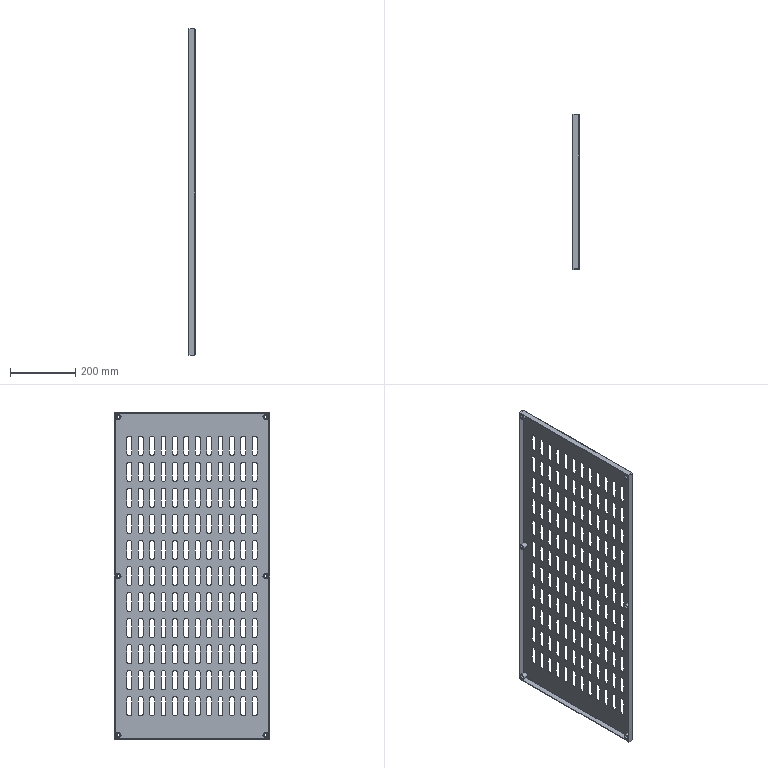Part | SolidWorks | 7 solids | 614 faces | box 19 x 477 x 1002 mm | volume 840276 mm3 | cylinder 308 | plane 302 | spline 4 | commonest cylinder face diameters 15 x264 9 x12 10 x12 16 x12 0.2 x4 4.2 x4